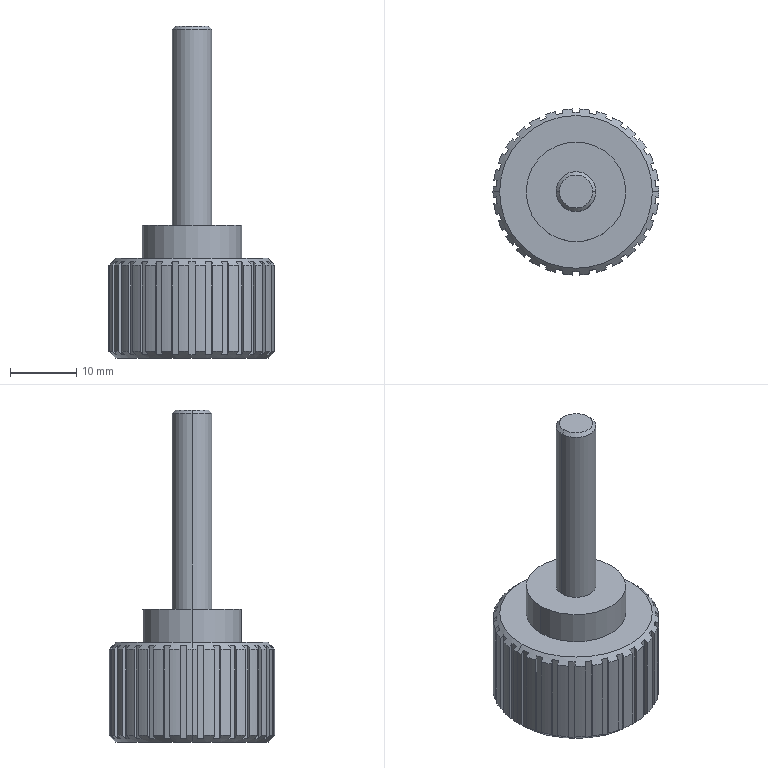Part | STEP file | M6 Bag feed screw | 1 solid | 135 faces | box 25 x 24.98 x 50 mm | volume 8815 mm3 | plane 94 | cylinder 35 | cone 6 | commonest cylinder face diameters 25 x31 6 x2 15 x2